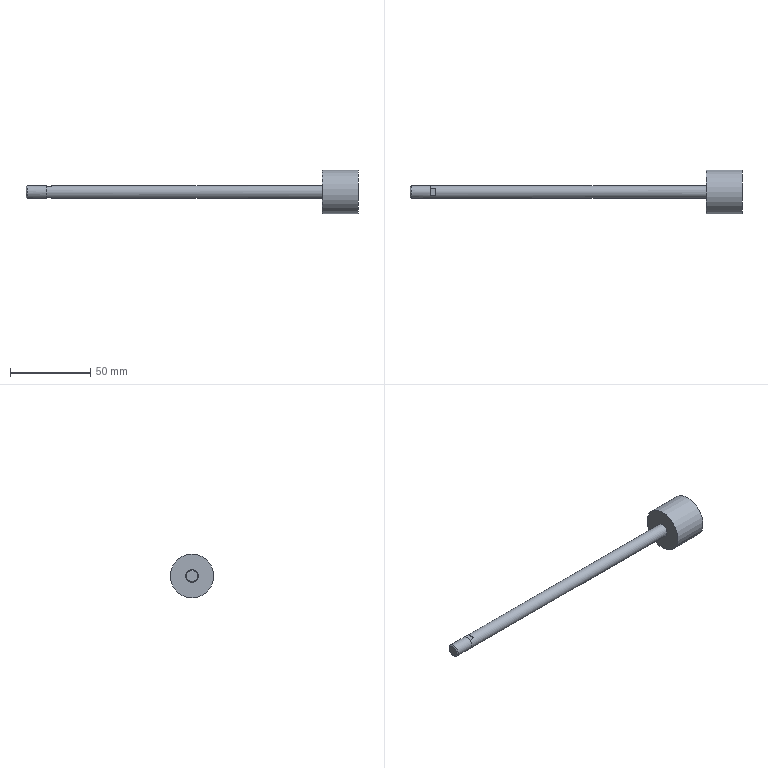Part | NX | features solid 2 | 1 solid | 13 faces | box 206.273 x 27.115 x 27.115 mm | volume 21841 mm3 | plane 9 | cylinder 3 | cone 1 | commonest cylinder face diameters 7.925 x1 7.938 x1 27.114 x1
STEP:
#1=CARTESIAN_POINT('',(-3.175,-2.376,3.175));
#2=VERTEX_POINT('',#1);
#3=CARTESIAN_POINT('',(0.,-2.371,3.175));
#4=VERTEX_POINT('',#3);
#5=CARTESIAN_POINT('',(190.398,-2.371,3.175));
#6=DIRECTION('',(-1.,0.,0.));
#7=VECTOR('',#6,1000.);
#8=LINE('',#5,#7);
#9=EDGE_CURVE('',#2,#4,#8,.F.);
#10=ORIENTED_EDGE('',*,*,#9,.F.);
#11=CARTESIAN_POINT('',(-3.175,-2.376,-3.175));
#12=VERTEX_POINT('',#11);
#13=CARTESIAN_POINT('',(-3.175,-2.374,3.172));
#14=CARTESIAN_POINT('',(-3.175,-3.356,2.438));
#15=CARTESIAN_POINT('',(-3.175,-4.569,0.));
#16=CARTESIAN_POINT('',(-3.175,-3.356,-2.438));
#17=CARTESIAN_POINT('',(-3.175,-2.374,-3.172));
#18=B_SPLINE_CURVE_WITH_KNOTS('',3,(#13,#14,#15,#16,#17),.UNSPECIFIED.,.F.,.F.,(4,1,4),(0.1022,0.25,0.3978),.UNSPECIFIED.);
#19=EDGE_CURVE('',#12,#2,#18,.F.);
#20=ORIENTED_EDGE('',*,*,#19,.F.);
#21=CARTESIAN_POINT('',(0.,-2.371,-3.175));
#22=VERTEX_POINT('',#21);
#23=CARTESIAN_POINT('',(190.398,-2.371,-3.175));
#24=DIRECTION('',(-1.,0.,0.));
#25=VECTOR('',#24,1000.);
#26=LINE('',#23,#25);
#27=EDGE_CURVE('',#22,#12,#26,.T.);
#28=ORIENTED_EDGE('',*,*,#27,.F.);
#29=CARTESIAN_POINT('',(0.,2.371,-3.175));
#30=VERTEX_POINT('',#29);
#31=CARTESIAN_POINT('',(0.,0.,0.));
#32=DIRECTION('',(1.,0.,0.));
#33=DIRECTION('',(0.,0.,-1.));
#34=AXIS2_PLACEMENT_3D('',#31,#32,#33);
#35=CIRCLE('',#34,3.962);
#36=EDGE_CURVE('',#30,#22,#35,.F.);
#37=ORIENTED_EDGE('',*,*,#36,.F.);
#38=CARTESIAN_POINT('',(-3.175,2.376,-3.175));
#39=VERTEX_POINT('',#38);
#40=CARTESIAN_POINT('',(190.398,2.371,-3.175));
#41=DIRECTION('',(-1.,0.,0.));
#42=VECTOR('',#41,1000.);
#43=LINE('',#40,#42);
#44=EDGE_CURVE('',#39,#30,#43,.F.);
#45=ORIENTED_EDGE('',*,*,#44,.F.);
#46=CARTESIAN_POINT('',(-3.175,2.376,3.175));
#47=VERTEX_POINT('',#46);
#48=CARTESIAN_POINT('',(-3.175,2.374,-3.172));
#49=CARTESIAN_POINT('',(-3.175,3.356,-2.438));
#50=CARTESIAN_POINT('',(-3.175,4.569,0.));
#51=CARTESIAN_POINT('',(-3.175,3.356,2.438));
#52=CARTESIAN_POINT('',(-3.175,2.374,3.172));
#53=B_SPLINE_CURVE_WITH_KNOTS('',3,(#48,#49,#50,#51,#52),.UNSPECIFIED.,.F.,.F.,(4,1,4),(0.6022,0.75,0.8978),.UNSPECIFIED.);
#54=EDGE_CURVE('',#47,#39,#53,.F.);
#55=ORIENTED_EDGE('',*,*,#54,.F.);
#56=CARTESIAN_POINT('',(0.,2.371,3.175));
#57=VERTEX_POINT('',#56);
#58=CARTESIAN_POINT('',(190.398,2.371,3.175));
#59=DIRECTION('',(-1.,0.,0.));
#60=VECTOR('',#59,1000.);
#61=LINE('',#58,#60);
#62=EDGE_CURVE('',#57,#47,#61,.T.);
#63=ORIENTED_EDGE('',*,*,#62,.F.);
#64=CARTESIAN_POINT('',(0.,0.,0.));
#65=DIRECTION('',(1.,0.,0.));
#66=DIRECTION('',(0.,0.,-1.));
#67=AXIS2_PLACEMENT_3D('',#64,#65,#66);
#68=CIRCLE('',#67,3.962);
#69=EDGE_CURVE('',#4,#57,#68,.F.);
#70=ORIENTED_EDGE('',*,*,#69,.F.);
#71=EDGE_LOOP('',(#10,#20,#28,#37,#45,#55,#63,#70));
#72=FACE_BOUND('',#71,.T.);
#73=CARTESIAN_POINT('',(168.275,0.,3.962));
#74=VERTEX_POINT('',#73);
#75=CARTESIAN_POINT('',(168.275,0.,0.));
#76=DIRECTION('',(-1.,0.,0.));
#77=DIRECTION('',(0.,0.,1.));
#78=AXIS2_PLACEMENT_3D('',#75,#76,#77);
#79=CIRCLE('',#78,3.962);
#80=EDGE_CURVE('',#74,#74,#79,.T.);
#81=ORIENTED_EDGE('',*,*,#80,.T.);
#82=EDGE_LOOP('',(#81));
#83=FACE_BOUND('',#82,.T.);
#84=CARTESIAN_POINT('',(190.398,0.,0.));
#85=DIRECTION('',(-1.,0.,0.));
#86=DIRECTION('',(0.,0.,1.));
#87=AXIS2_PLACEMENT_3D('',#84,#85,#86);
#88=CYLINDRICAL_SURFACE('',#87,3.962);
#89=ADVANCED_FACE('',(#72,#83),#88,.T.);
#90=CARTESIAN_POINT('',(168.275,0.,13.557));
#91=VERTEX_POINT('',#90);
#92=CARTESIAN_POINT('',(168.275,0.,0.));
#93=DIRECTION('',(-1.,0.,0.));
#94=DIRECTION('',(0.,0.,1.));
#95=AXIS2_PLACEMENT_3D('',#92,#93,#94);
#96=CIRCLE('',#95,13.557);
#97=EDGE_CURVE('',#91,#91,#96,.T.);
#98=ORIENTED_EDGE('',*,*,#97,.T.);
#99=EDGE_LOOP('',(#98));
#100=FACE_BOUND('',#99,.T.);
#101=ORIENTED_EDGE('',*,*,#80,.F.);
#102=EDGE_LOOP('',(#101));
#103=FACE_BOUND('',#102,.T.);
#104=CARTESIAN_POINT('',(168.275,3.962,0.));
#105=DIRECTION('',(-1.,0.,0.));
#106=DIRECTION('',(0.,0.,1.));
#107=AXIS2_PLACEMENT_3D('',#104,#105,#106);
#108=PLANE('',#107);
#109=ADVANCED_FACE('',(#100,#103),#108,.T.);
#110=CARTESIAN_POINT('',(190.398,0.,13.557));
#111=VERTEX_POINT('',#110);
#112=CARTESIAN_POINT('',(190.398,0.,0.));
#113=DIRECTION('',(-1.,0.,0.));
#114=DIRECTION('',(0.,0.,1.));
#115=AXIS2_PLACEMENT_3D('',#112,#113,#114);
#116=CIRCLE('',#115,13.557);
#117=EDGE_CURVE('',#111,#111,#116,.T.);
#118=ORIENTED_EDGE('',*,*,#117,.T.);
#119=EDGE_LOOP('',(#118));
#120=FACE_BOUND('',#119,.T.);
#121=ORIENTED_EDGE('',*,*,#97,.F.);
#122=EDGE_LOOP('',(#121));
#123=FACE_BOUND('',#122,.T.);
#124=CARTESIAN_POINT('',(190.398,0.,0.));
#125=DIRECTION('',(-1.,0.,0.));
#126=DIRECTION('',(0.,0.,1.));
#127=AXIS2_PLACEMENT_3D('',#124,#125,#126);
#128=CYLINDRICAL_SURFACE('',#127,13.557);
#129=ADVANCED_FACE('',(#120,#123),#128,.T.);
#130=ORIENTED_EDGE('',*,*,#117,.F.);
#131=EDGE_LOOP('',(#130));
#132=FACE_BOUND('',#131,.T.);
#133=CARTESIAN_POINT('',(190.398,13.557,0.));
#134=DIRECTION('',(1.,0.,0.));
#135=DIRECTION('',(0.,0.,-1.));
#136=AXIS2_PLACEMENT_3D('',#133,#134,#135);
#137=PLANE('',#136);
#138=ADVANCED_FACE('',(#132),#137,.T.);
#139=CARTESIAN_POINT('',(-15.245,0.,3.969));
#140=VERTEX_POINT('',#139);
#141=CARTESIAN_POINT('',(-15.245,0.,0.));
#142=DIRECTION('',(-1.,0.,0.));
#143=DIRECTION('',(0.,0.,1.));
#144=AXIS2_PLACEMENT_3D('',#141,#142,#143);
#145=CIRCLE('',#144,3.969);
#146=EDGE_CURVE('',#140,#140,#145,.T.);
#147=ORIENTED_EDGE('',*,*,#146,.T.);
#148=EDGE_LOOP('',(#147));
#149=FACE_BOUND('',#148,.T.);
#150=CARTESIAN_POINT('',(-15.875,0.,3.339));
#151=VERTEX_POINT('',#150);
#152=CARTESIAN_POINT('',(-15.875,0.,0.));
#153=DIRECTION('',(-1.,0.,0.));
#154=DIRECTION('',(0.,0.,1.));
#155=AXIS2_PLACEMENT_3D('',#152,#153,#154);
#156=CIRCLE('',#155,3.339);
#157=EDGE_CURVE('',#151,#151,#156,.T.);
#158=ORIENTED_EDGE('',*,*,#157,.F.);
#159=EDGE_LOOP('',(#158));
#160=FACE_BOUND('',#159,.T.);
#161=CARTESIAN_POINT('',(-15.875,0.,0.));
#162=DIRECTION('',(1.,0.,0.));
#163=DIRECTION('',(0.,0.,-1.));
#164=AXIS2_PLACEMENT_3D('',#161,#162,#163);
#165=CONICAL_SURFACE('',#164,3.339,0.7854);
#166=ADVANCED_FACE('',(#149,#160),#165,.T.);
#167=ORIENTED_EDGE('',*,*,#54,.T.);
#168=CARTESIAN_POINT('',(-3.175,2.381,-3.175));
#169=CARTESIAN_POINT('',(-3.175,1.006,-4.205));
#170=CARTESIAN_POINT('',(-3.175,-1.005,-4.207));
#171=CARTESIAN_POINT('',(-3.175,-2.381,-3.175));
#172=B_SPLINE_CURVE_WITH_KNOTS('',3,(#168,#169,#170,#171),.UNSPECIFIED.,.F.,.F.,(4,4),(0.,1.),.UNSPECIFIED.);
#173=EDGE_CURVE('',#39,#12,#172,.T.);
#174=ORIENTED_EDGE('',*,*,#173,.T.);
#175=ORIENTED_EDGE('',*,*,#19,.T.);
#176=CARTESIAN_POINT('',(-3.175,-2.381,3.175));
#177=CARTESIAN_POINT('',(-3.175,-1.006,4.205));
#178=CARTESIAN_POINT('',(-3.175,1.005,4.207));
#179=CARTESIAN_POINT('',(-3.175,2.381,3.175));
#180=B_SPLINE_CURVE_WITH_KNOTS('',3,(#176,#177,#178,#179),.UNSPECIFIED.,.F.,.F.,(4,4),(0.,1.),.UNSPECIFIED.);
#181=EDGE_CURVE('',#2,#47,#180,.T.);
#182=ORIENTED_EDGE('',*,*,#181,.T.);
#183=EDGE_LOOP('',(#167,#174,#175,#182));
#184=FACE_BOUND('',#183,.T.);
#185=ORIENTED_EDGE('',*,*,#146,.F.);
#186=EDGE_LOOP('',(#185));
#187=FACE_BOUND('',#186,.T.);
#188=CARTESIAN_POINT('',(-3.175,0.,0.));
#189=DIRECTION('',(-1.,0.,0.));
#190=DIRECTION('',(0.,0.,1.));
#191=AXIS2_PLACEMENT_3D('',#188,#189,#190);
#192=CYLINDRICAL_SURFACE('',#191,3.969);
#193=ADVANCED_FACE('',(#184,#187),#192,.T.);
#194=ORIENTED_EDGE('',*,*,#157,.T.);
#195=EDGE_LOOP('',(#194));
#196=FACE_BOUND('',#195,.T.);
#197=CARTESIAN_POINT('',(-15.875,0.,0.));
#198=DIRECTION('',(-1.,0.,0.));
#199=DIRECTION('',(0.,0.,1.));
#200=AXIS2_PLACEMENT_3D('',#197,#198,#199);
#201=PLANE('',#200);
#202=ADVANCED_FACE('',(#196),#201,.T.);
#203=ORIENTED_EDGE('',*,*,#36,.T.);
#204=CARTESIAN_POINT('',(0.,-3.962,-3.175));
#205=DIRECTION('',(0.,1.,0.));
#206=VECTOR('',#205,1000.);
#207=LINE('',#204,#206);
#208=EDGE_CURVE('',#22,#30,#207,.T.);
#209=ORIENTED_EDGE('',*,*,#208,.T.);
#210=EDGE_LOOP('',(#203,#209));
#211=FACE_BOUND('',#210,.T.);
#212=CARTESIAN_POINT('',(0.,7.925,-7.925));
#213=DIRECTION('',(1.,0.,0.));
#214=DIRECTION('',(0.,0.,-1.));
#215=AXIS2_PLACEMENT_3D('',#212,#213,#214);
#216=PLANE('',#215);
#217=ADVANCED_FACE('',(#211),#216,.F.);
#218=CARTESIAN_POINT('',(-3.175,-3.962,-3.175));
#219=DIRECTION('',(0.,1.,0.));
#220=VECTOR('',#219,1000.);
#221=LINE('',#218,#220);
#222=EDGE_CURVE('',#12,#39,#221,.T.);
#223=ORIENTED_EDGE('',*,*,#222,.F.);
#224=ORIENTED_EDGE('',*,*,#173,.F.);
#225=EDGE_LOOP('',(#223,#224));
#226=FACE_BOUND('',#225,.T.);
#227=CARTESIAN_POINT('',(-3.175,7.925,-7.925));
#228=DIRECTION('',(1.,0.,0.));
#229=DIRECTION('',(0.,0.,-1.));
#230=AXIS2_PLACEMENT_3D('',#227,#228,#229);
#231=PLANE('',#230);
#232=ADVANCED_FACE('',(#226),#231,.T.);
#233=ORIENTED_EDGE('',*,*,#44,.T.);
#234=ORIENTED_EDGE('',*,*,#208,.F.);
#235=ORIENTED_EDGE('',*,*,#27,.T.);
#236=ORIENTED_EDGE('',*,*,#222,.T.);
#237=EDGE_LOOP('',(#233,#234,#235,#236));
#238=FACE_BOUND('',#237,.T.);
#239=CARTESIAN_POINT('',(0.,-3.962,-3.175));
#240=DIRECTION('',(0.,0.,1.));
#241=DIRECTION('',(1.,0.,0.));
#242=AXIS2_PLACEMENT_3D('',#239,#240,#241);
#243=PLANE('',#242);
#244=ADVANCED_FACE('',(#238),#243,.F.);
#245=ORIENTED_EDGE('',*,*,#69,.T.);
#246=CARTESIAN_POINT('',(0.,3.962,3.175));
#247=DIRECTION('',(0.,-1.,0.));
#248=VECTOR('',#247,1000.);
#249=LINE('',#246,#248);
#250=EDGE_CURVE('',#57,#4,#249,.T.);
#251=ORIENTED_EDGE('',*,*,#250,.T.);
#252=EDGE_LOOP('',(#245,#251));
#253=FACE_BOUND('',#252,.T.);
#254=CARTESIAN_POINT('',(0.,7.925,-7.925));
#255=DIRECTION('',(1.,0.,0.));
#256=DIRECTION('',(0.,0.,-1.));
#257=AXIS2_PLACEMENT_3D('',#254,#255,#256);
#258=PLANE('',#257);
#259=ADVANCED_FACE('',(#253),#258,.F.);
#260=CARTESIAN_POINT('',(-3.175,3.962,3.175));
#261=DIRECTION('',(0.,-1.,0.));
#262=VECTOR('',#261,1000.);
#263=LINE('',#260,#262);
#264=EDGE_CURVE('',#47,#2,#263,.T.);
#265=ORIENTED_EDGE('',*,*,#264,.F.);
#266=ORIENTED_EDGE('',*,*,#181,.F.);
#267=EDGE_LOOP('',(#265,#266));
#268=FACE_BOUND('',#267,.T.);
#269=CARTESIAN_POINT('',(-3.175,7.925,-7.925));
#270=DIRECTION('',(1.,0.,0.));
#271=DIRECTION('',(0.,0.,-1.));
#272=AXIS2_PLACEMENT_3D('',#269,#270,#271);
#273=PLANE('',#272);
#274=ADVANCED_FACE('',(#268),#273,.T.);
#275=ORIENTED_EDGE('',*,*,#9,.T.);
#276=ORIENTED_EDGE('',*,*,#250,.F.);
#277=ORIENTED_EDGE('',*,*,#62,.T.);
#278=ORIENTED_EDGE('',*,*,#264,.T.);
#279=EDGE_LOOP('',(#275,#276,#277,#278));
#280=FACE_BOUND('',#279,.T.);
#281=CARTESIAN_POINT('',(0.,3.962,3.175));
#282=DIRECTION('',(0.,0.,-1.));
#283=DIRECTION('',(-1.,0.,0.));
#284=AXIS2_PLACEMENT_3D('',#281,#282,#283);
#285=PLANE('',#284);
#286=ADVANCED_FACE('',(#280),#285,.F.);
#287=CLOSED_SHELL('',(#89,#109,#129,#138,#166,#193,#202,#217,#232,#244,#259,#274,#286));
#288=MANIFOLD_SOLID_BREP('',#287);
#289=(LENGTH_UNIT()NAMED_UNIT(*)SI_UNIT(.MILLI.,.METRE.));
#290=UNCERTAINTY_MEASURE_WITH_UNIT(LENGTH_MEASURE(0.0508),#289,'','');
#291=(NAMED_UNIT(*)PLANE_ANGLE_UNIT()SI_UNIT($,.RADIAN.));
#292=(NAMED_UNIT(*)SI_UNIT($,.STERADIAN.)SOLID_ANGLE_UNIT());
#293=(GEOMETRIC_REPRESENTATION_CONTEXT(3)GLOBAL_UNCERTAINTY_ASSIGNED_CONTEXT((#290))GLOBAL_UNIT_ASSIGNED_CONTEXT((#289,#291,#292))REPRESENTATION_CONTEXT('',''));
#294=ADVANCED_BREP_SHAPE_REPRESENTATION('',(#288),#293);